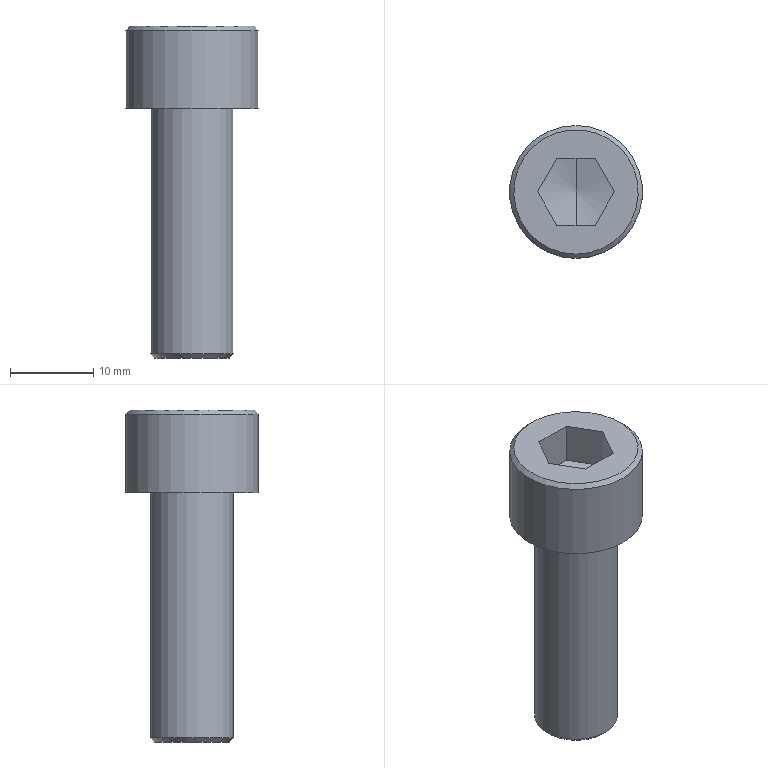Part | STEP file | 1_id4158_x_t | 1 solid | 21 faces | box 16 x 16 x 40 mm | volume 4057 mm3 | plane 15 | cone 4 | cylinder 2 | commonest cylinder face diameters 10 x1 16 x1
STEP:
#1=CARTESIAN_POINT('',(3849.5,-64.369,-17.));
#2=VERTEX_POINT('',#1);
#3=CARTESIAN_POINT('',(3849.5,-59.75,-18.));
#4=VERTEX_POINT('',#3);
#5=CARTESIAN_POINT('',(3849.5,-62.06,-17.5));
#6=DIRECTION('',(0.,0.9774,-0.2116));
#7=VECTOR('',#6,1.);
#8=LINE('',#5,#7);
#9=EDGE_CURVE('',#2,#4,#8,.T.);
#10=ORIENTED_EDGE('',*,*,#9,.F.);
#11=CARTESIAN_POINT('',(3851.81,-63.75,-17.));
#12=VERTEX_POINT('',#11);
#13=CARTESIAN_POINT('',(3849.5,-59.75,-17.));
#14=DIRECTION('',(0.,0.,-1.));
#15=DIRECTION('',(0.,1.,0.));
#16=AXIS2_PLACEMENT_3D('',#13,#14,#15);
#17=CIRCLE('',#16,4.619);
#18=EDGE_CURVE('',#12,#2,#17,.T.);
#19=ORIENTED_EDGE('',*,*,#18,.F.);
#20=CARTESIAN_POINT('',(3854.119,-59.75,-17.));
#21=VERTEX_POINT('',#20);
#22=CARTESIAN_POINT('',(3849.5,-59.75,-17.));
#23=DIRECTION('',(0.,0.,-1.));
#24=DIRECTION('',(0.,1.,0.));
#25=AXIS2_PLACEMENT_3D('',#22,#23,#24);
#26=CIRCLE('',#25,4.619);
#27=EDGE_CURVE('',#21,#12,#26,.T.);
#28=ORIENTED_EDGE('',*,*,#27,.F.);
#29=CARTESIAN_POINT('',(3851.81,-55.75,-17.));
#30=VERTEX_POINT('',#29);
#31=CARTESIAN_POINT('',(3849.5,-59.75,-17.));
#32=DIRECTION('',(0.,0.,-1.));
#33=DIRECTION('',(0.,1.,0.));
#34=AXIS2_PLACEMENT_3D('',#31,#32,#33);
#35=CIRCLE('',#34,4.619);
#36=EDGE_CURVE('',#30,#21,#35,.T.);
#37=ORIENTED_EDGE('',*,*,#36,.F.);
#38=CARTESIAN_POINT('',(3849.5,-55.131,-17.));
#39=VERTEX_POINT('',#38);
#40=CARTESIAN_POINT('',(3849.5,-59.75,-17.));
#41=DIRECTION('',(0.,0.,-1.));
#42=DIRECTION('',(0.,1.,0.));
#43=AXIS2_PLACEMENT_3D('',#40,#41,#42);
#44=CIRCLE('',#43,4.619);
#45=EDGE_CURVE('',#39,#30,#44,.T.);
#46=ORIENTED_EDGE('',*,*,#45,.F.);
#47=CARTESIAN_POINT('',(3849.5,-57.441,-17.5));
#48=DIRECTION('',(0.,0.9774,0.2116));
#49=VECTOR('',#48,1.);
#50=LINE('',#47,#49);
#51=EDGE_CURVE('',#4,#39,#50,.T.);
#52=ORIENTED_EDGE('',*,*,#51,.F.);
#53=EDGE_LOOP('',(#10,#19,#28,#37,#46,#52));
#54=FACE_OUTER_BOUND('',#53,.T.);
#55=CARTESIAN_POINT('',(3849.5,-59.75,-17.5));
#56=DIRECTION('',(0.,0.,1.));
#57=DIRECTION('',(0.,-1.,0.));
#58=AXIS2_PLACEMENT_3D('',#55,#56,#57);
#59=CONICAL_SURFACE('',#58,2.309,77.784);
#60=ADVANCED_FACE('',(#54),#59,.F.);
#61=CARTESIAN_POINT('',(3849.5,-64.75,-51.5));
#62=VERTEX_POINT('',#61);
#63=CARTESIAN_POINT('',(3849.5,-59.75,-51.5));
#64=DIRECTION('',(0.,0.,1.));
#65=DIRECTION('',(0.,-1.,0.));
#66=AXIS2_PLACEMENT_3D('',#63,#64,#65);
#67=CIRCLE('',#66,5.);
#68=EDGE_CURVE('',#62,#62,#67,.T.);
#69=ORIENTED_EDGE('',*,*,#68,.F.);
#70=EDGE_LOOP('',(#69));
#71=FACE_BOUND('',#70,.T.);
#72=CARTESIAN_POINT('',(3849.5,-64.25,-52.));
#73=VERTEX_POINT('',#72);
#74=CARTESIAN_POINT('',(3849.5,-59.75,-52.));
#75=DIRECTION('',(0.,0.,-1.));
#76=DIRECTION('',(0.,-1.,0.));
#77=AXIS2_PLACEMENT_3D('',#74,#75,#76);
#78=CIRCLE('',#77,4.5);
#79=EDGE_CURVE('',#73,#73,#78,.T.);
#80=ORIENTED_EDGE('',*,*,#79,.F.);
#81=EDGE_LOOP('',(#80));
#82=FACE_BOUND('',#81,.T.);
#83=CARTESIAN_POINT('',(3849.5,-59.75,-52.));
#84=DIRECTION('',(0.,0.,1.));
#85=DIRECTION('',(0.,1.,0.));
#86=AXIS2_PLACEMENT_3D('',#83,#84,#85);
#87=CONICAL_SURFACE('',#86,4.5,45.);
#88=ADVANCED_FACE('',(#71,#82),#87,.T.);
#89=ORIENTED_EDGE('',*,*,#68,.T.);
#90=EDGE_LOOP('',(#89));
#91=FACE_BOUND('',#90,.T.);
#92=CARTESIAN_POINT('',(3849.5,-54.75,-22.));
#93=VERTEX_POINT('',#92);
#94=CARTESIAN_POINT('',(3849.5,-59.75,-22.));
#95=DIRECTION('',(0.,0.,-1.));
#96=DIRECTION('',(0.,1.,0.));
#97=AXIS2_PLACEMENT_3D('',#94,#95,#96);
#98=CIRCLE('',#97,5.);
#99=EDGE_CURVE('',#93,#93,#98,.T.);
#100=ORIENTED_EDGE('',*,*,#99,.T.);
#101=EDGE_LOOP('',(#100));
#102=FACE_BOUND('',#101,.T.);
#103=CARTESIAN_POINT('',(3849.5,-59.75,-37.));
#104=DIRECTION('',(0.,0.,-1.));
#105=DIRECTION('',(0.,-1.,0.));
#106=AXIS2_PLACEMENT_3D('',#103,#104,#105);
#107=CYLINDRICAL_SURFACE('',#106,5.);
#108=ADVANCED_FACE('',(#91,#102),#107,.T.);
#109=ORIENTED_EDGE('',*,*,#79,.T.);
#110=EDGE_LOOP('',(#109));
#111=FACE_OUTER_BOUND('',#110,.T.);
#112=CARTESIAN_POINT('',(3849.5,-59.75,-52.));
#113=DIRECTION('',(0.,0.,-1.));
#114=DIRECTION('',(0.,-1.,0.));
#115=AXIS2_PLACEMENT_3D('',#112,#113,#114);
#116=PLANE('',#115);
#117=ADVANCED_FACE('',(#111),#116,.T.);
#118=CARTESIAN_POINT('',(3849.5,-67.25,-12.));
#119=VERTEX_POINT('',#118);
#120=CARTESIAN_POINT('',(3849.5,-59.75,-12.));
#121=DIRECTION('',(0.,0.,1.));
#122=DIRECTION('',(0.,-1.,0.));
#123=AXIS2_PLACEMENT_3D('',#120,#121,#122);
#124=CIRCLE('',#123,7.5);
#125=EDGE_CURVE('',#119,#119,#124,.T.);
#126=ORIENTED_EDGE('',*,*,#125,.F.);
#127=EDGE_LOOP('',(#126));
#128=FACE_BOUND('',#127,.T.);
#129=CARTESIAN_POINT('',(3849.5,-67.75,-12.5));
#130=VERTEX_POINT('',#129);
#131=CARTESIAN_POINT('',(3849.5,-59.75,-12.5));
#132=DIRECTION('',(0.,0.,-1.));
#133=DIRECTION('',(0.,-1.,0.));
#134=AXIS2_PLACEMENT_3D('',#131,#132,#133);
#135=CIRCLE('',#134,8.);
#136=EDGE_CURVE('',#130,#130,#135,.T.);
#137=ORIENTED_EDGE('',*,*,#136,.F.);
#138=EDGE_LOOP('',(#137));
#139=FACE_BOUND('',#138,.T.);
#140=CARTESIAN_POINT('',(3849.5,-59.75,-12.));
#141=DIRECTION('',(0.,0.,-1.));
#142=DIRECTION('',(0.,1.,0.));
#143=AXIS2_PLACEMENT_3D('',#140,#141,#142);
#144=CONICAL_SURFACE('',#143,7.5,45.);
#145=ADVANCED_FACE('',(#128,#139),#144,.T.);
#146=ORIENTED_EDGE('',*,*,#136,.T.);
#147=EDGE_LOOP('',(#146));
#148=FACE_BOUND('',#147,.T.);
#149=CARTESIAN_POINT('',(3849.5,-51.75,-22.));
#150=VERTEX_POINT('',#149);
#151=CARTESIAN_POINT('',(3849.5,-59.75,-22.));
#152=DIRECTION('',(0.,0.,1.));
#153=DIRECTION('',(0.,1.,0.));
#154=AXIS2_PLACEMENT_3D('',#151,#152,#153);
#155=CIRCLE('',#154,8.);
#156=EDGE_CURVE('',#150,#150,#155,.T.);
#157=ORIENTED_EDGE('',*,*,#156,.T.);
#158=EDGE_LOOP('',(#157));
#159=FACE_BOUND('',#158,.T.);
#160=CARTESIAN_POINT('',(3849.5,-59.75,-17.));
#161=DIRECTION('',(0.,0.,-1.));
#162=DIRECTION('',(0.,-1.,0.));
#163=AXIS2_PLACEMENT_3D('',#160,#161,#162);
#164=CYLINDRICAL_SURFACE('',#163,8.);
#165=ADVANCED_FACE('',(#148,#159),#164,.T.);
#166=CARTESIAN_POINT('',(3854.119,-59.75,-12.));
#167=VERTEX_POINT('',#166);
#168=CARTESIAN_POINT('',(3851.81,-55.75,-12.));
#169=VERTEX_POINT('',#168);
#170=CARTESIAN_POINT('',(3852.964,-57.75,-12.));
#171=DIRECTION('',(-0.5,0.866,0.));
#172=VECTOR('',#171,1.);
#173=LINE('',#170,#172);
#174=EDGE_CURVE('',#167,#169,#173,.T.);
#175=ORIENTED_EDGE('',*,*,#174,.F.);
#176=CARTESIAN_POINT('',(3851.81,-63.75,-12.));
#177=VERTEX_POINT('',#176);
#178=CARTESIAN_POINT('',(3852.964,-61.75,-12.));
#179=DIRECTION('',(0.5,0.866,0.));
#180=VECTOR('',#179,1.);
#181=LINE('',#178,#180);
#182=EDGE_CURVE('',#177,#167,#181,.T.);
#183=ORIENTED_EDGE('',*,*,#182,.F.);
#184=CARTESIAN_POINT('',(3847.191,-63.75,-12.));
#185=VERTEX_POINT('',#184);
#186=CARTESIAN_POINT('',(3849.5,-63.75,-12.));
#187=DIRECTION('',(1.,0.,0.));
#188=VECTOR('',#187,1.);
#189=LINE('',#186,#188);
#190=EDGE_CURVE('',#185,#177,#189,.T.);
#191=ORIENTED_EDGE('',*,*,#190,.F.);
#192=CARTESIAN_POINT('',(3844.881,-59.75,-12.));
#193=VERTEX_POINT('',#192);
#194=CARTESIAN_POINT('',(3846.036,-61.75,-12.));
#195=DIRECTION('',(0.5,-0.866,0.));
#196=VECTOR('',#195,1.);
#197=LINE('',#194,#196);
#198=EDGE_CURVE('',#193,#185,#197,.T.);
#199=ORIENTED_EDGE('',*,*,#198,.F.);
#200=CARTESIAN_POINT('',(3847.191,-55.75,-12.));
#201=VERTEX_POINT('',#200);
#202=CARTESIAN_POINT('',(3846.036,-57.75,-12.));
#203=DIRECTION('',(-0.5,-0.866,0.));
#204=VECTOR('',#203,1.);
#205=LINE('',#202,#204);
#206=EDGE_CURVE('',#201,#193,#205,.T.);
#207=ORIENTED_EDGE('',*,*,#206,.F.);
#208=CARTESIAN_POINT('',(3849.5,-55.75,-12.));
#209=DIRECTION('',(-1.,0.,0.));
#210=VECTOR('',#209,1.);
#211=LINE('',#208,#210);
#212=EDGE_CURVE('',#169,#201,#211,.T.);
#213=ORIENTED_EDGE('',*,*,#212,.F.);
#214=EDGE_LOOP('',(#175,#183,#191,#199,#207,#213));
#215=FACE_BOUND('',#214,.T.);
#216=ORIENTED_EDGE('',*,*,#125,.T.);
#217=EDGE_LOOP('',(#216));
#218=FACE_BOUND('',#217,.T.);
#219=CARTESIAN_POINT('',(3849.5,-59.75,-12.));
#220=DIRECTION('',(0.,0.,1.));
#221=DIRECTION('',(0.,1.,0.));
#222=AXIS2_PLACEMENT_3D('',#219,#220,#221);
#223=PLANE('',#222);
#224=ADVANCED_FACE('',(#215,#218),#223,.T.);
#225=CARTESIAN_POINT('',(3852.964,-57.75,-17.));
#226=DIRECTION('',(-0.5,0.866,0.));
#227=VECTOR('',#226,1.);
#228=LINE('',#225,#227);
#229=EDGE_CURVE('',#21,#30,#228,.T.);
#230=ORIENTED_EDGE('',*,*,#229,.T.);
#231=ORIENTED_EDGE('',*,*,#36,.T.);
#232=EDGE_LOOP('',(#230,#231));
#233=FACE_OUTER_BOUND('',#232,.T.);
#234=CARTESIAN_POINT('',(3849.5,-59.75,-17.));
#235=DIRECTION('',(0.,0.,1.));
#236=DIRECTION('',(0.,1.,0.));
#237=AXIS2_PLACEMENT_3D('',#234,#235,#236);
#238=PLANE('',#237);
#239=ADVANCED_FACE('',(#233),#238,.F.);
#240=CARTESIAN_POINT('',(3847.191,-55.75,-17.));
#241=VERTEX_POINT('',#240);
#242=CARTESIAN_POINT('',(3849.5,-55.75,-17.));
#243=DIRECTION('',(-1.,0.,0.));
#244=VECTOR('',#243,1.);
#245=LINE('',#242,#244);
#246=EDGE_CURVE('',#30,#241,#245,.T.);
#247=ORIENTED_EDGE('',*,*,#246,.T.);
#248=CARTESIAN_POINT('',(3849.5,-59.75,-17.));
#249=DIRECTION('',(0.,0.,-1.));
#250=DIRECTION('',(0.,1.,0.));
#251=AXIS2_PLACEMENT_3D('',#248,#249,#250);
#252=CIRCLE('',#251,4.619);
#253=EDGE_CURVE('',#241,#39,#252,.T.);
#254=ORIENTED_EDGE('',*,*,#253,.T.);
#255=ORIENTED_EDGE('',*,*,#45,.T.);
#256=EDGE_LOOP('',(#247,#254,#255));
#257=FACE_OUTER_BOUND('',#256,.T.);
#258=CARTESIAN_POINT('',(3849.5,-59.75,-17.));
#259=DIRECTION('',(0.,0.,1.));
#260=DIRECTION('',(0.,1.,0.));
#261=AXIS2_PLACEMENT_3D('',#258,#259,#260);
#262=PLANE('',#261);
#263=ADVANCED_FACE('',(#257),#262,.F.);
#264=CARTESIAN_POINT('',(3844.881,-59.75,-17.));
#265=VERTEX_POINT('',#264);
#266=CARTESIAN_POINT('',(3846.036,-57.75,-17.));
#267=DIRECTION('',(-0.5,-0.866,0.));
#268=VECTOR('',#267,1.);
#269=LINE('',#266,#268);
#270=EDGE_CURVE('',#241,#265,#269,.T.);
#271=ORIENTED_EDGE('',*,*,#270,.T.);
#272=CARTESIAN_POINT('',(3849.5,-59.75,-17.));
#273=DIRECTION('',(0.,0.,-1.));
#274=DIRECTION('',(0.,1.,0.));
#275=AXIS2_PLACEMENT_3D('',#272,#273,#274);
#276=CIRCLE('',#275,4.619);
#277=EDGE_CURVE('',#265,#241,#276,.T.);
#278=ORIENTED_EDGE('',*,*,#277,.T.);
#279=EDGE_LOOP('',(#271,#278));
#280=FACE_OUTER_BOUND('',#279,.T.);
#281=CARTESIAN_POINT('',(3849.5,-59.75,-17.));
#282=DIRECTION('',(0.,0.,1.));
#283=DIRECTION('',(0.,1.,0.));
#284=AXIS2_PLACEMENT_3D('',#281,#282,#283);
#285=PLANE('',#284);
#286=ADVANCED_FACE('',(#280),#285,.F.);
#287=CARTESIAN_POINT('',(3847.191,-63.75,-17.));
#288=VERTEX_POINT('',#287);
#289=CARTESIAN_POINT('',(3846.036,-61.75,-17.));
#290=DIRECTION('',(0.5,-0.866,0.));
#291=VECTOR('',#290,1.);
#292=LINE('',#289,#291);
#293=EDGE_CURVE('',#265,#288,#292,.T.);
#294=ORIENTED_EDGE('',*,*,#293,.T.);
#295=CARTESIAN_POINT('',(3849.5,-59.75,-17.));
#296=DIRECTION('',(0.,0.,-1.));
#297=DIRECTION('',(0.,1.,0.));
#298=AXIS2_PLACEMENT_3D('',#295,#296,#297);
#299=CIRCLE('',#298,4.619);
#300=EDGE_CURVE('',#288,#265,#299,.T.);
#301=ORIENTED_EDGE('',*,*,#300,.T.);
#302=EDGE_LOOP('',(#294,#301));
#303=FACE_OUTER_BOUND('',#302,.T.);
#304=CARTESIAN_POINT('',(3849.5,-59.75,-17.));
#305=DIRECTION('',(0.,0.,1.));
#306=DIRECTION('',(0.,1.,0.));
#307=AXIS2_PLACEMENT_3D('',#304,#305,#306);
#308=PLANE('',#307);
#309=ADVANCED_FACE('',(#303),#308,.F.);
#310=CARTESIAN_POINT('',(3849.5,-63.75,-17.));
#311=DIRECTION('',(1.,0.,0.));
#312=VECTOR('',#311,1.);
#313=LINE('',#310,#312);
#314=EDGE_CURVE('',#288,#12,#313,.T.);
#315=ORIENTED_EDGE('',*,*,#314,.T.);
#316=ORIENTED_EDGE('',*,*,#18,.T.);
#317=CARTESIAN_POINT('',(3849.5,-59.75,-17.));
#318=DIRECTION('',(0.,0.,-1.));
#319=DIRECTION('',(0.,1.,0.));
#320=AXIS2_PLACEMENT_3D('',#317,#318,#319);
#321=CIRCLE('',#320,4.619);
#322=EDGE_CURVE('',#2,#288,#321,.T.);
#323=ORIENTED_EDGE('',*,*,#322,.T.);
#324=EDGE_LOOP('',(#315,#316,#323));
#325=FACE_OUTER_BOUND('',#324,.T.);
#326=CARTESIAN_POINT('',(3849.5,-59.75,-17.));
#327=DIRECTION('',(0.,0.,1.));
#328=DIRECTION('',(0.,1.,0.));
#329=AXIS2_PLACEMENT_3D('',#326,#327,#328);
#330=PLANE('',#329);
#331=ADVANCED_FACE('',(#325),#330,.F.);
#332=CARTESIAN_POINT('',(3852.964,-61.75,-17.));
#333=DIRECTION('',(0.5,0.866,0.));
#334=VECTOR('',#333,1.);
#335=LINE('',#332,#334);
#336=EDGE_CURVE('',#12,#21,#335,.T.);
#337=ORIENTED_EDGE('',*,*,#336,.T.);
#338=ORIENTED_EDGE('',*,*,#27,.T.);
#339=EDGE_LOOP('',(#337,#338));
#340=FACE_OUTER_BOUND('',#339,.T.);
#341=CARTESIAN_POINT('',(3849.5,-59.75,-17.));
#342=DIRECTION('',(0.,0.,1.));
#343=DIRECTION('',(0.,1.,0.));
#344=AXIS2_PLACEMENT_3D('',#341,#342,#343);
#345=PLANE('',#344);
#346=ADVANCED_FACE('',(#340),#345,.F.);
#347=ORIENTED_EDGE('',*,*,#9,.T.);
#348=ORIENTED_EDGE('',*,*,#51,.T.);
#349=ORIENTED_EDGE('',*,*,#253,.F.);
#350=ORIENTED_EDGE('',*,*,#277,.F.);
#351=ORIENTED_EDGE('',*,*,#300,.F.);
#352=ORIENTED_EDGE('',*,*,#322,.F.);
#353=EDGE_LOOP('',(#347,#348,#349,#350,#351,#352));
#354=FACE_OUTER_BOUND('',#353,.T.);
#355=CARTESIAN_POINT('',(3849.5,-59.75,-17.5));
#356=DIRECTION('',(0.,0.,1.));
#357=DIRECTION('',(0.,-1.,0.));
#358=AXIS2_PLACEMENT_3D('',#355,#356,#357);
#359=CONICAL_SURFACE('',#358,2.309,77.784);
#360=ADVANCED_FACE('',(#354),#359,.F.);
#361=CARTESIAN_POINT('',(3854.119,-59.75,-14.5));
#362=DIRECTION('',(0.,0.,1.));
#363=VECTOR('',#362,1.);
#364=LINE('',#361,#363);
#365=EDGE_CURVE('',#21,#167,#364,.T.);
#366=ORIENTED_EDGE('',*,*,#365,.T.);
#367=ORIENTED_EDGE('',*,*,#174,.T.);
#368=CARTESIAN_POINT('',(3851.81,-55.75,-14.5));
#369=DIRECTION('',(0.,0.,1.));
#370=VECTOR('',#369,1.);
#371=LINE('',#368,#370);
#372=EDGE_CURVE('',#30,#169,#371,.T.);
#373=ORIENTED_EDGE('',*,*,#372,.F.);
#374=ORIENTED_EDGE('',*,*,#229,.F.);
#375=EDGE_LOOP('',(#366,#367,#373,#374));
#376=FACE_OUTER_BOUND('',#375,.T.);
#377=CARTESIAN_POINT('',(3852.964,-57.75,-14.5));
#378=DIRECTION('',(-0.866,-0.5,0.));
#379=DIRECTION('',(0.,0.,1.));
#380=AXIS2_PLACEMENT_3D('',#377,#378,#379);
#381=PLANE('',#380);
#382=ADVANCED_FACE('',(#376),#381,.T.);
#383=CARTESIAN_POINT('',(3851.81,-63.75,-14.5));
#384=DIRECTION('',(0.,0.,1.));
#385=VECTOR('',#384,1.);
#386=LINE('',#383,#385);
#387=EDGE_CURVE('',#12,#177,#386,.T.);
#388=ORIENTED_EDGE('',*,*,#387,.T.);
#389=ORIENTED_EDGE('',*,*,#182,.T.);
#390=ORIENTED_EDGE('',*,*,#365,.F.);
#391=ORIENTED_EDGE('',*,*,#336,.F.);
#392=EDGE_LOOP('',(#388,#389,#390,#391));
#393=FACE_OUTER_BOUND('',#392,.T.);
#394=CARTESIAN_POINT('',(3852.964,-61.75,-14.5));
#395=DIRECTION('',(-0.866,0.5,0.));
#396=DIRECTION('',(0.,0.,-1.));
#397=AXIS2_PLACEMENT_3D('',#394,#395,#396);
#398=PLANE('',#397);
#399=ADVANCED_FACE('',(#393),#398,.T.);
#400=CARTESIAN_POINT('',(3847.191,-63.75,-14.5));
#401=DIRECTION('',(0.,0.,1.));
#402=VECTOR('',#401,1.);
#403=LINE('',#400,#402);
#404=EDGE_CURVE('',#288,#185,#403,.T.);
#405=ORIENTED_EDGE('',*,*,#404,.T.);
#406=ORIENTED_EDGE('',*,*,#190,.T.);
#407=ORIENTED_EDGE('',*,*,#387,.F.);
#408=ORIENTED_EDGE('',*,*,#314,.F.);
#409=EDGE_LOOP('',(#405,#406,#407,#408));
#410=FACE_OUTER_BOUND('',#409,.T.);
#411=CARTESIAN_POINT('',(3849.5,-63.75,-14.5));
#412=DIRECTION('',(0.,1.,0.));
#413=DIRECTION('',(0.,0.,-1.));
#414=AXIS2_PLACEMENT_3D('',#411,#412,#413);
#415=PLANE('',#414);
#416=ADVANCED_FACE('',(#410),#415,.T.);
#417=CARTESIAN_POINT('',(3844.881,-59.75,-14.5));
#418=DIRECTION('',(0.,0.,1.));
#419=VECTOR('',#418,1.);
#420=LINE('',#417,#419);
#421=EDGE_CURVE('',#265,#193,#420,.T.);
#422=ORIENTED_EDGE('',*,*,#421,.T.);
#423=ORIENTED_EDGE('',*,*,#198,.T.);
#424=ORIENTED_EDGE('',*,*,#404,.F.);
#425=ORIENTED_EDGE('',*,*,#293,.F.);
#426=EDGE_LOOP('',(#422,#423,#424,#425));
#427=FACE_OUTER_BOUND('',#426,.T.);
#428=CARTESIAN_POINT('',(3846.036,-61.75,-14.5));
#429=DIRECTION('',(0.866,0.5,0.));
#430=DIRECTION('',(0.,0.,-1.));
#431=AXIS2_PLACEMENT_3D('',#428,#429,#430);
#432=PLANE('',#431);
#433=ADVANCED_FACE('',(#427),#432,.T.);
#434=CARTESIAN_POINT('',(3847.191,-55.75,-14.5));
#435=DIRECTION('',(0.,0.,1.));
#436=VECTOR('',#435,1.);
#437=LINE('',#434,#436);
#438=EDGE_CURVE('',#241,#201,#437,.T.);
#439=ORIENTED_EDGE('',*,*,#438,.T.);
#440=ORIENTED_EDGE('',*,*,#206,.T.);
#441=ORIENTED_EDGE('',*,*,#421,.F.);
#442=ORIENTED_EDGE('',*,*,#270,.F.);
#443=EDGE_LOOP('',(#439,#440,#441,#442));
#444=FACE_OUTER_BOUND('',#443,.T.);
#445=CARTESIAN_POINT('',(3846.036,-57.75,-14.5));
#446=DIRECTION('',(0.866,-0.5,0.));
#447=DIRECTION('',(0.,0.,1.));
#448=AXIS2_PLACEMENT_3D('',#445,#446,#447);
#449=PLANE('',#448);
#450=ADVANCED_FACE('',(#444),#449,.T.);
#451=ORIENTED_EDGE('',*,*,#372,.T.);
#452=ORIENTED_EDGE('',*,*,#212,.T.);
#453=ORIENTED_EDGE('',*,*,#438,.F.);
#454=ORIENTED_EDGE('',*,*,#246,.F.);
#455=EDGE_LOOP('',(#451,#452,#453,#454));
#456=FACE_OUTER_BOUND('',#455,.T.);
#457=CARTESIAN_POINT('',(3849.5,-55.75,-14.5));
#458=DIRECTION('',(0.,-1.,0.));
#459=DIRECTION('',(0.,0.,1.));
#460=AXIS2_PLACEMENT_3D('',#457,#458,#459);
#461=PLANE('',#460);
#462=ADVANCED_FACE('',(#456),#461,.T.);
#463=ORIENTED_EDGE('',*,*,#99,.F.);
#464=EDGE_LOOP('',(#463));
#465=FACE_BOUND('',#464,.T.);
#466=ORIENTED_EDGE('',*,*,#156,.F.);
#467=EDGE_LOOP('',(#466));
#468=FACE_BOUND('',#467,.T.);
#469=CARTESIAN_POINT('',(3849.5,-59.75,-22.));
#470=DIRECTION('',(0.,0.,-1.));
#471=DIRECTION('',(0.,-1.,0.));
#472=AXIS2_PLACEMENT_3D('',#469,#470,#471);
#473=PLANE('',#472);
#474=ADVANCED_FACE('',(#465,#468),#473,.T.);
#475=CLOSED_SHELL('',(#60,#88,#108,#117,#145,#165,#224,#239,#263,#286,#309,#331,#346,#360,#382,#399,#416,#433,#450,#462,#474));
#476=MANIFOLD_SOLID_BREP('',#475);
#477=(LENGTH_UNIT()NAMED_UNIT(*)SI_UNIT(.MILLI.,.METRE.));
#478=UNCERTAINTY_MEASURE_WITH_UNIT(LENGTH_MEASURE(0.00002),#477,'','');
#479=(NAMED_UNIT(*)PLANE_ANGLE_UNIT()SI_UNIT($,.RADIAN.));
#480=PLANE_ANGLE_MEASURE_WITH_UNIT(PLANE_ANGLE_MEASURE(0.01745),#479);
#481=DIMENSIONAL_EXPONENTS(0.,0.,0.,0.,0.,0.,0.);
#482=(CONVERSION_BASED_UNIT('DEGREE',#480)NAMED_UNIT(#481)PLANE_ANGLE_UNIT());
#483=(NAMED_UNIT(*)SI_UNIT($,.STERADIAN.)SOLID_ANGLE_UNIT());
#484=(GEOMETRIC_REPRESENTATION_CONTEXT(3)GLOBAL_UNCERTAINTY_ASSIGNED_CONTEXT((#478))GLOBAL_UNIT_ASSIGNED_CONTEXT((#477,#482,#483))REPRESENTATION_CONTEXT('',''));
#485=ADVANCED_BREP_SHAPE_REPRESENTATION('',(#476),#484);